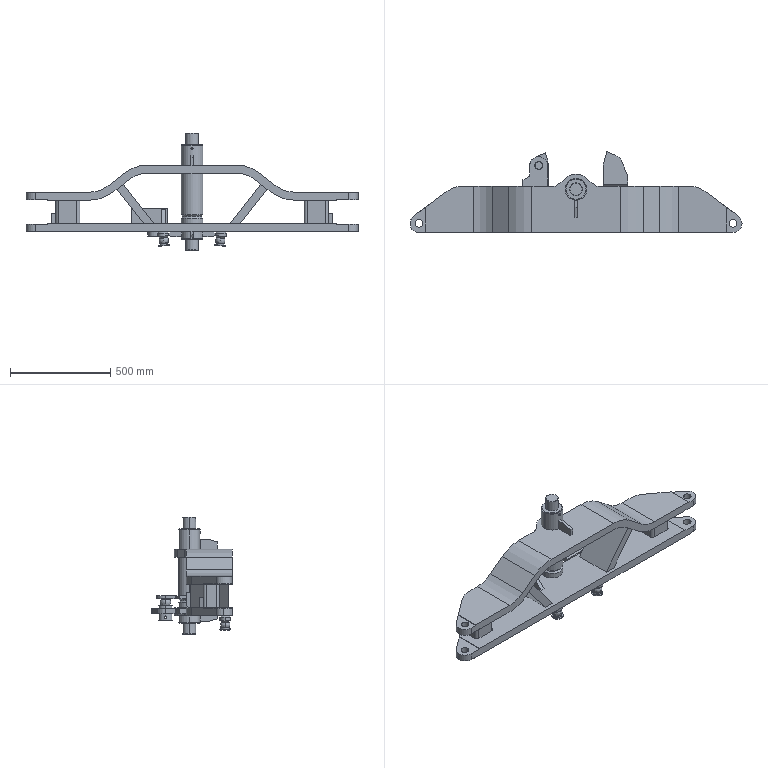Part | SolidWorks | 32 solids | 412 faces | box 1658 x 403.509 x 586 mm | volume 38283555 mm3 | plane 194 | cylinder 150 | cone 54 | sphere 6 | spline 4 | torus 4 | commonest cylinder face diameters 12 x16 40 x16 90 x15 108 x10 7 x8 9 x8